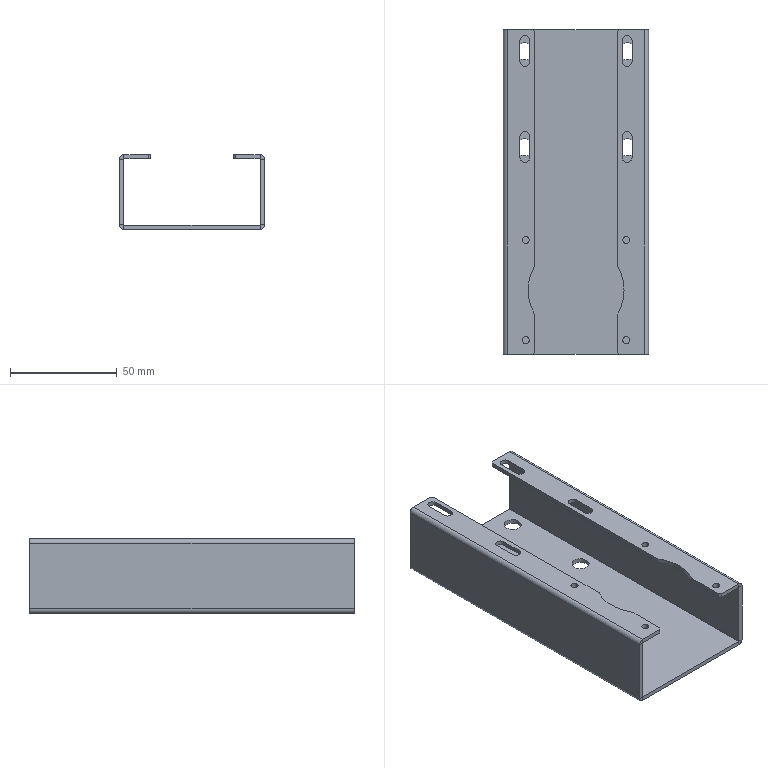Part | STEP file | Motor fixing plate 2 | 1 solid | 79 faces | box 68 x 152 x 35 mm | volume 46618 mm3 | plane 44 | cylinder 35 | commonest cylinder face diameters 3.3 x8 4.5 x8 8 x8 0.2 x4 4.2 x4 45 x3